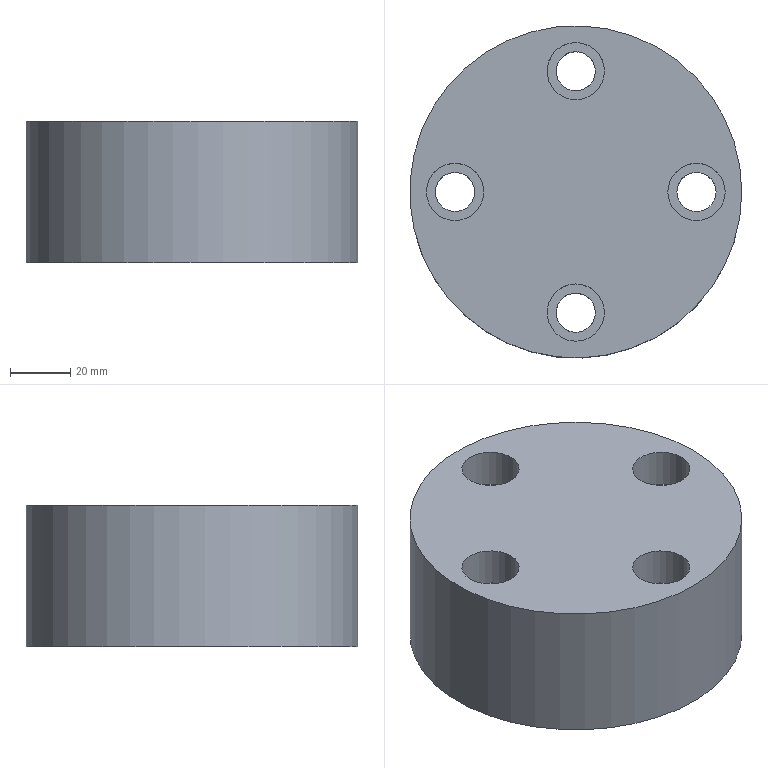CAM job | NX | 3-axis milling, drilling | part box 110 x 110 x 47 mm | stock box 110 x 110 x 47 mm
Tools:
number,name,description,diameter,corner_radius,flute_length,length,flutes
1,ZXZ,Milling Tool-5 Parameters,6.0,0.0,50.0,75.0,2
3,13.0ZT,Drilling Tool,13.0,0.0,35.0,50.0,2
10,D10,Milling Tool-5 Parameters,10.0,0.0,50.0,75.0,2
7,D6A45,Milling Tool-5 Parameters,6.0,0.0,50.0,75.0,2
Operations:
program,operation,operation_type,tool,method,geometry_group,spindle_rpm,surface_speed,feed_per_tooth,feed_cut,feed_plunge,cut_length_mm,path_length_mm,cut_time_min,machine_time_min
1,DRILLING,Operation,ZXZ,METHOD,A,3500.0,65.0,0.0357,250.0,0.0,16.0,270.944,0.064,0.0895
1,DRILLING_COPY_COPY,Operation,13.0ZT,METHOD,A,500.0,20.0,0.15,150.0,0.0,221.622,682.189,1.478,1.524
1,HOLE_MILLING,CylinderMilling,D10,METHOD,A,3000.0,94.0,0.3667,2200.0,100.0,7109.92,7569.626,3.232,3.278
1,PLANAR_MILL,PlanarMilling,D6A45,METHOD,A,7500.0,141.0,0.0833,1250.0,100.0,257.81,635.66,0.2062,0.244